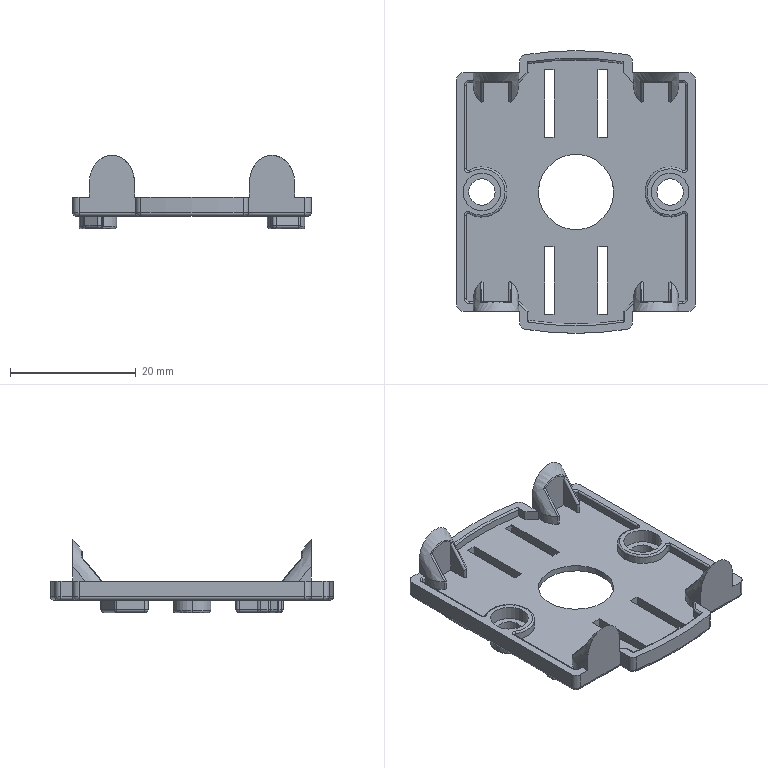Part | STEP file | PCS-02B-3_1_2.stp | 1 solid | 300 faces | box 38 x 45.04 x 11.674 mm | volume 2792 mm3 | cylinder 137 | plane 105 | sphere 23 | torus 19 | spline 16 | commonest cylinder face diameters 1 x60 0.6 x38 2 x8 6 x8 7.2 x8 4.2 x4